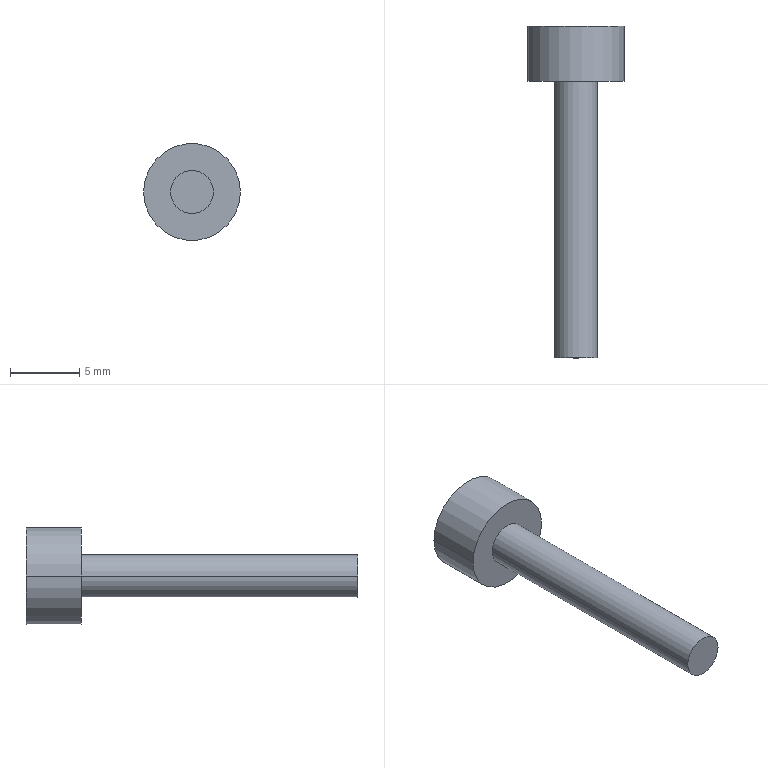Part | CATIA | 1 solid | 7 faces | box 7 x 24 x 7 mm | volume 304.892 mm3 | cylinder 4 | plane 3 | commonest cylinder face diameters 3.1 x2 7 x2
STEP:
#1=CARTESIAN_POINT('',(-24.,7.,16.5));
#2=VERTEX_POINT('',#1);
#3=CARTESIAN_POINT('',(-31.,7.,16.5));
#4=VERTEX_POINT('',#3);
#5=CARTESIAN_POINT('',(-27.5,7.,16.5));
#6=DIRECTION('',(0.,-1.,0.));
#7=AXIS2_PLACEMENT_3D('',#5,#6,$);
#8=CIRCLE('',#7,3.5);
#9=EDGE_CURVE('',#2,#4,#8,.F.);
#10=ORIENTED_EDGE('',*,*,#9,.F.);
#11=CARTESIAN_POINT('',(-27.5,7.,16.5));
#12=DIRECTION('',(0.,-1.,0.));
#13=AXIS2_PLACEMENT_3D('',#11,#12,$);
#14=CIRCLE('',#13,3.5);
#15=EDGE_CURVE('',#4,#2,#14,.F.);
#16=ORIENTED_EDGE('',*,*,#15,.F.);
#17=EDGE_LOOP('',(#10,#16));
#18=FACE_OUTER_BOUND('',#17,.T.);
#19=CARTESIAN_POINT('',(-25.95,7.,16.5));
#20=VERTEX_POINT('',#19);
#21=CARTESIAN_POINT('',(-29.05,7.,16.5));
#22=VERTEX_POINT('',#21);
#23=CARTESIAN_POINT('',(-27.5,7.,16.5));
#24=DIRECTION('',(0.,-1.,0.));
#25=AXIS2_PLACEMENT_3D('',#23,#24,$);
#26=CIRCLE('',#25,1.55);
#27=EDGE_CURVE('',#20,#22,#26,.T.);
#28=ORIENTED_EDGE('',*,*,#27,.F.);
#29=CARTESIAN_POINT('',(-27.5,7.,16.5));
#30=DIRECTION('',(0.,-1.,0.));
#31=AXIS2_PLACEMENT_3D('',#29,#30,$);
#32=CIRCLE('',#31,1.55);
#33=EDGE_CURVE('',#22,#20,#32,.T.);
#34=ORIENTED_EDGE('',*,*,#33,.F.);
#35=EDGE_LOOP('',(#28,#34));
#36=FACE_BOUND('',#35,.T.);
#37=CARTESIAN_POINT('',(0.,7.,0.));
#38=DIRECTION('',(0.,-1.,0.));
#39=DIRECTION('',(1.,0.,0.));
#40=AXIS2_PLACEMENT_3D('',#37,#38,#39);
#41=PLANE('',#40);
#42=ADVANCED_FACE('',(#18,#36),#41,.T.);
#43=CARTESIAN_POINT('',(-24.,11.,16.5));
#44=VERTEX_POINT('',#43);
#45=CARTESIAN_POINT('',(-24.,9.,16.5));
#46=DIRECTION('',(0.,1.,0.));
#47=VECTOR('',#46,1.);
#48=LINE('',#45,#47);
#49=EDGE_CURVE('',#2,#44,#48,.T.);
#50=ORIENTED_EDGE('',*,*,#49,.F.);
#51=ORIENTED_EDGE('',*,*,#9,.T.);
#52=CARTESIAN_POINT('',(-31.,11.,16.5));
#53=VERTEX_POINT('',#52);
#54=CARTESIAN_POINT('',(-31.,9.,16.5));
#55=DIRECTION('',(0.,1.,0.));
#56=VECTOR('',#55,1.);
#57=LINE('',#54,#56);
#58=EDGE_CURVE('',#4,#53,#57,.T.);
#59=ORIENTED_EDGE('',*,*,#58,.T.);
#60=CARTESIAN_POINT('',(-27.5,11.,16.5));
#61=DIRECTION('',(0.,1.,0.));
#62=AXIS2_PLACEMENT_3D('',#60,#61,$);
#63=CIRCLE('',#62,3.5);
#64=EDGE_CURVE('',#44,#53,#63,.T.);
#65=ORIENTED_EDGE('',*,*,#64,.F.);
#66=EDGE_LOOP('',(#50,#51,#59,#65));
#67=FACE_OUTER_BOUND('',#66,.T.);
#68=CARTESIAN_POINT('',(-27.5,9.,16.5));
#69=DIRECTION('',(0.,1.,0.));
#70=DIRECTION('',(1.,0.,0.));
#71=AXIS2_PLACEMENT_3D('',#68,#69,#70);
#72=CYLINDRICAL_SURFACE('',#71,3.5);
#73=ADVANCED_FACE('',(#67),#72,.T.);
#74=ORIENTED_EDGE('',*,*,#58,.F.);
#75=ORIENTED_EDGE('',*,*,#15,.T.);
#76=ORIENTED_EDGE('',*,*,#49,.T.);
#77=CARTESIAN_POINT('',(-27.5,11.,16.5));
#78=DIRECTION('',(0.,1.,0.));
#79=AXIS2_PLACEMENT_3D('',#77,#78,$);
#80=CIRCLE('',#79,3.5);
#81=EDGE_CURVE('',#53,#44,#80,.T.);
#82=ORIENTED_EDGE('',*,*,#81,.F.);
#83=EDGE_LOOP('',(#74,#75,#76,#82));
#84=FACE_OUTER_BOUND('',#83,.T.);
#85=CARTESIAN_POINT('',(-27.5,9.,16.5));
#86=DIRECTION('',(0.,1.,0.));
#87=DIRECTION('',(-1.,0.,0.));
#88=AXIS2_PLACEMENT_3D('',#85,#86,#87);
#89=CYLINDRICAL_SURFACE('',#88,3.5);
#90=ADVANCED_FACE('',(#84),#89,.T.);
#91=CARTESIAN_POINT('',(-25.95,-13.,16.5));
#92=VERTEX_POINT('',#91);
#93=CARTESIAN_POINT('',(-25.95,-3.,16.5));
#94=DIRECTION('',(0.,-1.,0.));
#95=VECTOR('',#94,1.);
#96=LINE('',#93,#95);
#97=EDGE_CURVE('',#20,#92,#96,.T.);
#98=ORIENTED_EDGE('',*,*,#97,.F.);
#99=ORIENTED_EDGE('',*,*,#27,.T.);
#100=CARTESIAN_POINT('',(-29.05,-13.,16.5));
#101=VERTEX_POINT('',#100);
#102=CARTESIAN_POINT('',(-29.05,-3.,16.5));
#103=DIRECTION('',(0.,-1.,0.));
#104=VECTOR('',#103,1.);
#105=LINE('',#102,#104);
#106=EDGE_CURVE('',#22,#101,#105,.T.);
#107=ORIENTED_EDGE('',*,*,#106,.T.);
#108=CARTESIAN_POINT('',(-27.5,-13.,16.5));
#109=DIRECTION('',(0.,-1.,0.));
#110=AXIS2_PLACEMENT_3D('',#108,#109,$);
#111=CIRCLE('',#110,1.55);
#112=EDGE_CURVE('',#92,#101,#111,.T.);
#113=ORIENTED_EDGE('',*,*,#112,.F.);
#114=EDGE_LOOP('',(#98,#99,#107,#113));
#115=FACE_OUTER_BOUND('',#114,.T.);
#116=CARTESIAN_POINT('',(-27.5,-3.,16.5));
#117=DIRECTION('',(0.,-1.,0.));
#118=DIRECTION('',(1.,0.,0.));
#119=AXIS2_PLACEMENT_3D('',#116,#117,#118);
#120=CYLINDRICAL_SURFACE('',#119,1.55);
#121=ADVANCED_FACE('',(#115),#120,.T.);
#122=ORIENTED_EDGE('',*,*,#106,.F.);
#123=ORIENTED_EDGE('',*,*,#33,.T.);
#124=ORIENTED_EDGE('',*,*,#97,.T.);
#125=CARTESIAN_POINT('',(-27.5,-13.,16.5));
#126=DIRECTION('',(0.,-1.,0.));
#127=AXIS2_PLACEMENT_3D('',#125,#126,$);
#128=CIRCLE('',#127,1.55);
#129=EDGE_CURVE('',#101,#92,#128,.T.);
#130=ORIENTED_EDGE('',*,*,#129,.F.);
#131=EDGE_LOOP('',(#122,#123,#124,#130));
#132=FACE_OUTER_BOUND('',#131,.T.);
#133=CARTESIAN_POINT('',(-27.5,-3.,16.5));
#134=DIRECTION('',(0.,-1.,0.));
#135=DIRECTION('',(-1.,0.,0.));
#136=AXIS2_PLACEMENT_3D('',#133,#134,#135);
#137=CYLINDRICAL_SURFACE('',#136,1.55);
#138=ADVANCED_FACE('',(#132),#137,.T.);
#139=ORIENTED_EDGE('',*,*,#81,.T.);
#140=ORIENTED_EDGE('',*,*,#64,.T.);
#141=EDGE_LOOP('',(#139,#140));
#142=FACE_OUTER_BOUND('',#141,.T.);
#143=CARTESIAN_POINT('',(0.,11.,0.));
#144=DIRECTION('',(0.,1.,0.));
#145=DIRECTION('',(-1.,0.,0.));
#146=AXIS2_PLACEMENT_3D('',#143,#144,#145);
#147=PLANE('',#146);
#148=ADVANCED_FACE('',(#142),#147,.T.);
#149=ORIENTED_EDGE('',*,*,#112,.T.);
#150=ORIENTED_EDGE('',*,*,#129,.T.);
#151=EDGE_LOOP('',(#149,#150));
#152=FACE_OUTER_BOUND('',#151,.T.);
#153=CARTESIAN_POINT('',(0.,-13.,0.));
#154=DIRECTION('',(0.,-1.,0.));
#155=DIRECTION('',(1.,0.,0.));
#156=AXIS2_PLACEMENT_3D('',#153,#154,#155);
#157=PLANE('',#156);
#158=ADVANCED_FACE('',(#152),#157,.T.);
#159=CLOSED_SHELL('',(#42,#73,#90,#121,#138,#148,#158));
#160=MANIFOLD_SOLID_BREP('',#159);
#161=(LENGTH_UNIT()NAMED_UNIT(*)SI_UNIT(.MILLI.,.METRE.));
#162=UNCERTAINTY_MEASURE_WITH_UNIT(LENGTH_MEASURE(0.005),#161,'','');
#163=(NAMED_UNIT(*)PLANE_ANGLE_UNIT()SI_UNIT($,.RADIAN.));
#164=(NAMED_UNIT(*)SI_UNIT($,.STERADIAN.)SOLID_ANGLE_UNIT());
#165=(GEOMETRIC_REPRESENTATION_CONTEXT(3)GLOBAL_UNCERTAINTY_ASSIGNED_CONTEXT((#162))GLOBAL_UNIT_ASSIGNED_CONTEXT((#161,#163,#164))REPRESENTATION_CONTEXT('',''));
#166=ADVANCED_BREP_SHAPE_REPRESENTATION('',(#160),#165);